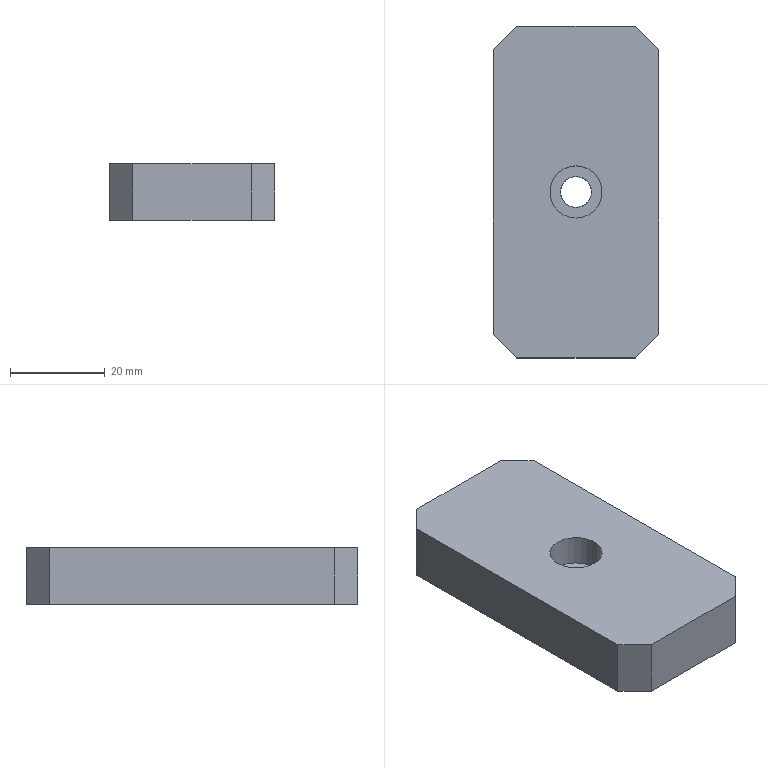Part | STEP file | P011002NM03-000 | 1 solid | 13 faces | box 35 x 70 x 12 mm | volume 28000 mm3 | plane 11 | cylinder 2 | commonest cylinder face diameters 6.5 x1 11 x1
STEP:
#1=CARTESIAN_POINT('',(0.,0.,0.));
#2=DIRECTION('',(0.,0.,1.));
#3=DIRECTION('',(1.,0.,0.));
#4=AXIS2_PLACEMENT_3D('',#1,#2,#3);
#5=CARTESIAN_POINT('',(-207.5,157.5,9.));
#6=VERTEX_POINT('',#5);
#7=CARTESIAN_POINT('',(-232.5,157.5,9.));
#8=VERTEX_POINT('',#7);
#9=CARTESIAN_POINT('',(-220.,157.5,9.));
#10=DIRECTION('',(-1.,0.,0.));
#11=VECTOR('',#10,1.);
#12=LINE('',#9,#11);
#13=CARTESIAN_POINT('',(-220.,157.5,6.));
#14=DIRECTION('',(0.,-1.,0.));
#15=DIRECTION('',(0.,0.,-1.));
#16=AXIS2_PLACEMENT_3D('',#13,#14,#15);
#17=PLANE('',#16);
#18=CARTESIAN_POINT('',(-3.,0.));
#19=DIRECTION('',(0.,-1.));
#20=VECTOR('',#19,1.);
#21=LINE('',#18,#20);
#22=(GEOMETRIC_REPRESENTATION_CONTEXT(2)PARAMETRIC_REPRESENTATION_CONTEXT()REPRESENTATION_CONTEXT('',''));
#23=DEFINITIONAL_REPRESENTATION('',(#21),#22);
#24=PCURVE('',#17,#23);
#25=CARTESIAN_POINT('',(178.,-325.,9.));
#26=DIRECTION('',(0.,0.,1.));
#27=DIRECTION('',(1.,0.,0.));
#28=AXIS2_PLACEMENT_3D('',#25,#26,#27);
#29=PLANE('',#28);
#30=CARTESIAN_POINT('',(-398.,482.5));
#31=DIRECTION('',(-1.,0.));
#32=VECTOR('',#31,1.);
#33=LINE('',#30,#32);
#34=(GEOMETRIC_REPRESENTATION_CONTEXT(2)PARAMETRIC_REPRESENTATION_CONTEXT()REPRESENTATION_CONTEXT('',''));
#35=DEFINITIONAL_REPRESENTATION('',(#33),#34);
#36=PCURVE('',#29,#35);
#37=SURFACE_CURVE('',#12,(#24,#36),.PCURVE_S1.);
#38=EDGE_CURVE('',#6,#8,#37,.T.);
#39=ORIENTED_EDGE('',*,*,#38,.F.);
#40=CARTESIAN_POINT('',(-207.5,157.5,21.));
#41=VERTEX_POINT('',#40);
#42=CARTESIAN_POINT('',(-207.5,157.5,6.));
#43=DIRECTION('',(0.,0.,1.));
#44=VECTOR('',#43,1.);
#45=LINE('',#42,#44);
#46=CARTESIAN_POINT('',(0.,12.5));
#47=DIRECTION('',(-1.,0.));
#48=VECTOR('',#47,1.);
#49=LINE('',#46,#48);
#50=(GEOMETRIC_REPRESENTATION_CONTEXT(2)PARAMETRIC_REPRESENTATION_CONTEXT()REPRESENTATION_CONTEXT('',''));
#51=DEFINITIONAL_REPRESENTATION('',(#49),#50);
#52=PCURVE('',#17,#51);
#53=CARTESIAN_POINT('',(-202.5,162.5,6.));
#54=DIRECTION('',(-0.7071,0.7071,0.));
#55=DIRECTION('',(-0.7071,-0.7071,0.));
#56=AXIS2_PLACEMENT_3D('',#53,#54,#55);
#57=PLANE('',#56);
#58=CARTESIAN_POINT('',(7.071,0.));
#59=DIRECTION('',(0.,1.));
#60=VECTOR('',#59,1.);
#61=LINE('',#58,#60);
#62=(GEOMETRIC_REPRESENTATION_CONTEXT(2)PARAMETRIC_REPRESENTATION_CONTEXT()REPRESENTATION_CONTEXT('',''));
#63=DEFINITIONAL_REPRESENTATION('',(#61),#62);
#64=PCURVE('',#57,#63);
#65=SURFACE_CURVE('',#45,(#52,#64),.PCURVE_S1.);
#66=EDGE_CURVE('',#6,#41,#65,.T.);
#67=ORIENTED_EDGE('',*,*,#66,.T.);
#68=CARTESIAN_POINT('',(-232.5,157.5,21.));
#69=VERTEX_POINT('',#68);
#70=CARTESIAN_POINT('',(-220.,157.5,21.));
#71=DIRECTION('',(-1.,0.,0.));
#72=VECTOR('',#71,1.);
#73=LINE('',#70,#72);
#74=CARTESIAN_POINT('',(-15.,0.));
#75=DIRECTION('',(0.,-1.));
#76=VECTOR('',#75,1.);
#77=LINE('',#74,#76);
#78=(GEOMETRIC_REPRESENTATION_CONTEXT(2)PARAMETRIC_REPRESENTATION_CONTEXT()REPRESENTATION_CONTEXT('',''));
#79=DEFINITIONAL_REPRESENTATION('',(#77),#78);
#80=PCURVE('',#17,#79);
#81=CARTESIAN_POINT('',(-205.,185.,21.));
#82=DIRECTION('',(0.,0.,1.));
#83=DIRECTION('',(1.,0.,0.));
#84=AXIS2_PLACEMENT_3D('',#81,#82,#83);
#85=PLANE('',#84);
#86=CARTESIAN_POINT('',(-15.,-27.5));
#87=DIRECTION('',(-1.,0.));
#88=VECTOR('',#87,1.);
#89=LINE('',#86,#88);
#90=(GEOMETRIC_REPRESENTATION_CONTEXT(2)PARAMETRIC_REPRESENTATION_CONTEXT()REPRESENTATION_CONTEXT('',''));
#91=DEFINITIONAL_REPRESENTATION('',(#89),#90);
#92=PCURVE('',#85,#91);
#93=SURFACE_CURVE('',#73,(#80,#92),.PCURVE_S1.);
#94=EDGE_CURVE('',#41,#69,#93,.T.);
#95=ORIENTED_EDGE('',*,*,#94,.T.);
#96=CARTESIAN_POINT('',(-232.5,157.5,6.));
#97=DIRECTION('',(0.,0.,-1.));
#98=VECTOR('',#97,1.);
#99=LINE('',#96,#98);
#100=CARTESIAN_POINT('',(0.,-12.5));
#101=DIRECTION('',(1.,0.));
#102=VECTOR('',#101,1.);
#103=LINE('',#100,#102);
#104=(GEOMETRIC_REPRESENTATION_CONTEXT(2)PARAMETRIC_REPRESENTATION_CONTEXT()REPRESENTATION_CONTEXT('',''));
#105=DEFINITIONAL_REPRESENTATION('',(#103),#104);
#106=PCURVE('',#17,#105);
#107=CARTESIAN_POINT('',(-232.5,157.5,6.));
#108=DIRECTION('',(0.7071,0.7071,0.));
#109=DIRECTION('',(-0.7071,0.7071,0.));
#110=AXIS2_PLACEMENT_3D('',#107,#108,#109);
#111=PLANE('',#110);
#112=CARTESIAN_POINT('',(0.,0.));
#113=DIRECTION('',(0.,-1.));
#114=VECTOR('',#113,1.);
#115=LINE('',#112,#114);
#116=(GEOMETRIC_REPRESENTATION_CONTEXT(2)PARAMETRIC_REPRESENTATION_CONTEXT()REPRESENTATION_CONTEXT('',''));
#117=DEFINITIONAL_REPRESENTATION('',(#115),#116);
#118=PCURVE('',#111,#117);
#119=SURFACE_CURVE('',#99,(#106,#118),.PCURVE_S1.);
#120=EDGE_CURVE('',#69,#8,#119,.T.);
#121=ORIENTED_EDGE('',*,*,#120,.T.);
#122=EDGE_LOOP('',(#39,#67,#95,#121));
#123=FACE_BOUND('',#122,.T.);
#124=ADVANCED_FACE('',(#123),#17,.T.);
#125=CARTESIAN_POINT('',(-202.5,222.5,9.));
#126=VERTEX_POINT('',#125);
#127=CARTESIAN_POINT('',(-202.5,162.5,9.));
#128=VERTEX_POINT('',#127);
#129=CARTESIAN_POINT('',(-202.5,192.5,9.));
#130=DIRECTION('',(0.,-1.,0.));
#131=VECTOR('',#130,1.);
#132=LINE('',#129,#131);
#133=CARTESIAN_POINT('',(-202.5,192.5,6.));
#134=DIRECTION('',(1.,0.,0.));
#135=DIRECTION('',(0.,0.,-1.));
#136=AXIS2_PLACEMENT_3D('',#133,#134,#135);
#137=PLANE('',#136);
#138=CARTESIAN_POINT('',(-3.,0.));
#139=DIRECTION('',(0.,-1.));
#140=VECTOR('',#139,1.);
#141=LINE('',#138,#140);
#142=(GEOMETRIC_REPRESENTATION_CONTEXT(2)PARAMETRIC_REPRESENTATION_CONTEXT()REPRESENTATION_CONTEXT('',''));
#143=DEFINITIONAL_REPRESENTATION('',(#141),#142);
#144=PCURVE('',#137,#143);
#145=CARTESIAN_POINT('',(-380.5,517.5));
#146=DIRECTION('',(0.,-1.));
#147=VECTOR('',#146,1.);
#148=LINE('',#145,#147);
#149=(GEOMETRIC_REPRESENTATION_CONTEXT(2)PARAMETRIC_REPRESENTATION_CONTEXT()REPRESENTATION_CONTEXT('',''));
#150=DEFINITIONAL_REPRESENTATION('',(#148),#149);
#151=PCURVE('',#29,#150);
#152=SURFACE_CURVE('',#132,(#144,#151),.PCURVE_S1.);
#153=EDGE_CURVE('',#126,#128,#152,.T.);
#154=ORIENTED_EDGE('',*,*,#153,.F.);
#155=CARTESIAN_POINT('',(-202.5,222.5,21.));
#156=VERTEX_POINT('',#155);
#157=CARTESIAN_POINT('',(-202.5,222.5,6.));
#158=DIRECTION('',(0.,0.,1.));
#159=VECTOR('',#158,1.);
#160=LINE('',#157,#159);
#161=CARTESIAN_POINT('',(0.,30.));
#162=DIRECTION('',(-1.,0.));
#163=VECTOR('',#162,1.);
#164=LINE('',#161,#163);
#165=(GEOMETRIC_REPRESENTATION_CONTEXT(2)PARAMETRIC_REPRESENTATION_CONTEXT()REPRESENTATION_CONTEXT('',''));
#166=DEFINITIONAL_REPRESENTATION('',(#164),#165);
#167=PCURVE('',#137,#166);
#168=CARTESIAN_POINT('',(-207.5,227.5,6.));
#169=DIRECTION('',(-0.7071,-0.7071,0.));
#170=DIRECTION('',(0.7071,-0.7071,0.));
#171=AXIS2_PLACEMENT_3D('',#168,#169,#170);
#172=PLANE('',#171);
#173=CARTESIAN_POINT('',(7.071,0.));
#174=DIRECTION('',(0.,1.));
#175=VECTOR('',#174,1.);
#176=LINE('',#173,#175);
#177=(GEOMETRIC_REPRESENTATION_CONTEXT(2)PARAMETRIC_REPRESENTATION_CONTEXT()REPRESENTATION_CONTEXT('',''));
#178=DEFINITIONAL_REPRESENTATION('',(#176),#177);
#179=PCURVE('',#172,#178);
#180=SURFACE_CURVE('',#160,(#167,#179),.PCURVE_S1.);
#181=EDGE_CURVE('',#126,#156,#180,.T.);
#182=ORIENTED_EDGE('',*,*,#181,.T.);
#183=CARTESIAN_POINT('',(-202.5,162.5,21.));
#184=VERTEX_POINT('',#183);
#185=CARTESIAN_POINT('',(-202.5,192.5,21.));
#186=DIRECTION('',(0.,-1.,0.));
#187=VECTOR('',#186,1.);
#188=LINE('',#185,#187);
#189=CARTESIAN_POINT('',(-15.,0.));
#190=DIRECTION('',(0.,-1.));
#191=VECTOR('',#190,1.);
#192=LINE('',#189,#191);
#193=(GEOMETRIC_REPRESENTATION_CONTEXT(2)PARAMETRIC_REPRESENTATION_CONTEXT()REPRESENTATION_CONTEXT('',''));
#194=DEFINITIONAL_REPRESENTATION('',(#192),#193);
#195=PCURVE('',#137,#194);
#196=CARTESIAN_POINT('',(2.5,7.5));
#197=DIRECTION('',(0.,-1.));
#198=VECTOR('',#197,1.);
#199=LINE('',#196,#198);
#200=(GEOMETRIC_REPRESENTATION_CONTEXT(2)PARAMETRIC_REPRESENTATION_CONTEXT()REPRESENTATION_CONTEXT('',''));
#201=DEFINITIONAL_REPRESENTATION('',(#199),#200);
#202=PCURVE('',#85,#201);
#203=SURFACE_CURVE('',#188,(#195,#202),.PCURVE_S1.);
#204=EDGE_CURVE('',#156,#184,#203,.T.);
#205=ORIENTED_EDGE('',*,*,#204,.T.);
#206=CARTESIAN_POINT('',(-202.5,162.5,6.));
#207=DIRECTION('',(0.,0.,-1.));
#208=VECTOR('',#207,1.);
#209=LINE('',#206,#208);
#210=CARTESIAN_POINT('',(0.,-30.));
#211=DIRECTION('',(1.,0.));
#212=VECTOR('',#211,1.);
#213=LINE('',#210,#212);
#214=(GEOMETRIC_REPRESENTATION_CONTEXT(2)PARAMETRIC_REPRESENTATION_CONTEXT()REPRESENTATION_CONTEXT('',''));
#215=DEFINITIONAL_REPRESENTATION('',(#213),#214);
#216=PCURVE('',#137,#215);
#217=CARTESIAN_POINT('',(0.,0.));
#218=DIRECTION('',(0.,-1.));
#219=VECTOR('',#218,1.);
#220=LINE('',#217,#219);
#221=(GEOMETRIC_REPRESENTATION_CONTEXT(2)PARAMETRIC_REPRESENTATION_CONTEXT()REPRESENTATION_CONTEXT('',''));
#222=DEFINITIONAL_REPRESENTATION('',(#220),#221);
#223=PCURVE('',#57,#222);
#224=SURFACE_CURVE('',#209,(#216,#223),.PCURVE_S1.);
#225=EDGE_CURVE('',#184,#128,#224,.T.);
#226=ORIENTED_EDGE('',*,*,#225,.T.);
#227=EDGE_LOOP('',(#154,#182,#205,#226));
#228=FACE_BOUND('',#227,.T.);
#229=ADVANCED_FACE('',(#228),#137,.T.);
#230=CARTESIAN_POINT('',(-232.5,227.5,9.));
#231=VERTEX_POINT('',#230);
#232=CARTESIAN_POINT('',(-207.5,227.5,9.));
#233=VERTEX_POINT('',#232);
#234=CARTESIAN_POINT('',(-220.,227.5,9.));
#235=DIRECTION('',(1.,0.,0.));
#236=VECTOR('',#235,1.);
#237=LINE('',#234,#236);
#238=CARTESIAN_POINT('',(-220.,227.5,6.));
#239=DIRECTION('',(0.,1.,0.));
#240=DIRECTION('',(0.,0.,1.));
#241=AXIS2_PLACEMENT_3D('',#238,#239,#240);
#242=PLANE('',#241);
#243=CARTESIAN_POINT('',(3.,0.));
#244=DIRECTION('',(0.,1.));
#245=VECTOR('',#244,1.);
#246=LINE('',#243,#245);
#247=(GEOMETRIC_REPRESENTATION_CONTEXT(2)PARAMETRIC_REPRESENTATION_CONTEXT()REPRESENTATION_CONTEXT('',''));
#248=DEFINITIONAL_REPRESENTATION('',(#246),#247);
#249=PCURVE('',#242,#248);
#250=CARTESIAN_POINT('',(-398.,552.5));
#251=DIRECTION('',(1.,0.));
#252=VECTOR('',#251,1.);
#253=LINE('',#250,#252);
#254=(GEOMETRIC_REPRESENTATION_CONTEXT(2)PARAMETRIC_REPRESENTATION_CONTEXT()REPRESENTATION_CONTEXT('',''));
#255=DEFINITIONAL_REPRESENTATION('',(#253),#254);
#256=PCURVE('',#29,#255);
#257=SURFACE_CURVE('',#237,(#249,#256),.PCURVE_S1.);
#258=EDGE_CURVE('',#231,#233,#257,.T.);
#259=ORIENTED_EDGE('',*,*,#258,.F.);
#260=CARTESIAN_POINT('',(-232.5,227.5,21.));
#261=VERTEX_POINT('',#260);
#262=CARTESIAN_POINT('',(-232.5,227.5,6.));
#263=DIRECTION('',(0.,0.,1.));
#264=VECTOR('',#263,1.);
#265=LINE('',#262,#264);
#266=CARTESIAN_POINT('',(0.,-12.5));
#267=DIRECTION('',(1.,0.));
#268=VECTOR('',#267,1.);
#269=LINE('',#266,#268);
#270=(GEOMETRIC_REPRESENTATION_CONTEXT(2)PARAMETRIC_REPRESENTATION_CONTEXT()REPRESENTATION_CONTEXT('',''));
#271=DEFINITIONAL_REPRESENTATION('',(#269),#270);
#272=PCURVE('',#242,#271);
#273=CARTESIAN_POINT('',(-237.5,222.5,6.));
#274=DIRECTION('',(0.7071,-0.7071,0.));
#275=DIRECTION('',(0.7071,0.7071,0.));
#276=AXIS2_PLACEMENT_3D('',#273,#274,#275);
#277=PLANE('',#276);
#278=CARTESIAN_POINT('',(7.071,0.));
#279=DIRECTION('',(0.,1.));
#280=VECTOR('',#279,1.);
#281=LINE('',#278,#280);
#282=(GEOMETRIC_REPRESENTATION_CONTEXT(2)PARAMETRIC_REPRESENTATION_CONTEXT()REPRESENTATION_CONTEXT('',''));
#283=DEFINITIONAL_REPRESENTATION('',(#281),#282);
#284=PCURVE('',#277,#283);
#285=SURFACE_CURVE('',#265,(#272,#284),.PCURVE_S1.);
#286=EDGE_CURVE('',#231,#261,#285,.T.);
#287=ORIENTED_EDGE('',*,*,#286,.T.);
#288=CARTESIAN_POINT('',(-207.5,227.5,21.));
#289=VERTEX_POINT('',#288);
#290=CARTESIAN_POINT('',(-220.,227.5,21.));
#291=DIRECTION('',(1.,0.,0.));
#292=VECTOR('',#291,1.);
#293=LINE('',#290,#292);
#294=CARTESIAN_POINT('',(15.,0.));
#295=DIRECTION('',(0.,1.));
#296=VECTOR('',#295,1.);
#297=LINE('',#294,#296);
#298=(GEOMETRIC_REPRESENTATION_CONTEXT(2)PARAMETRIC_REPRESENTATION_CONTEXT()REPRESENTATION_CONTEXT('',''));
#299=DEFINITIONAL_REPRESENTATION('',(#297),#298);
#300=PCURVE('',#242,#299);
#301=CARTESIAN_POINT('',(-15.,42.5));
#302=DIRECTION('',(1.,0.));
#303=VECTOR('',#302,1.);
#304=LINE('',#301,#303);
#305=(GEOMETRIC_REPRESENTATION_CONTEXT(2)PARAMETRIC_REPRESENTATION_CONTEXT()REPRESENTATION_CONTEXT('',''));
#306=DEFINITIONAL_REPRESENTATION('',(#304),#305);
#307=PCURVE('',#85,#306);
#308=SURFACE_CURVE('',#293,(#300,#307),.PCURVE_S1.);
#309=EDGE_CURVE('',#261,#289,#308,.T.);
#310=ORIENTED_EDGE('',*,*,#309,.T.);
#311=CARTESIAN_POINT('',(-207.5,227.5,6.));
#312=DIRECTION('',(0.,0.,-1.));
#313=VECTOR('',#312,1.);
#314=LINE('',#311,#313);
#315=CARTESIAN_POINT('',(0.,12.5));
#316=DIRECTION('',(-1.,0.));
#317=VECTOR('',#316,1.);
#318=LINE('',#315,#317);
#319=(GEOMETRIC_REPRESENTATION_CONTEXT(2)PARAMETRIC_REPRESENTATION_CONTEXT()REPRESENTATION_CONTEXT('',''));
#320=DEFINITIONAL_REPRESENTATION('',(#318),#319);
#321=PCURVE('',#242,#320);
#322=CARTESIAN_POINT('',(0.,0.));
#323=DIRECTION('',(0.,-1.));
#324=VECTOR('',#323,1.);
#325=LINE('',#322,#324);
#326=(GEOMETRIC_REPRESENTATION_CONTEXT(2)PARAMETRIC_REPRESENTATION_CONTEXT()REPRESENTATION_CONTEXT('',''));
#327=DEFINITIONAL_REPRESENTATION('',(#325),#326);
#328=PCURVE('',#172,#327);
#329=SURFACE_CURVE('',#314,(#321,#328),.PCURVE_S1.);
#330=EDGE_CURVE('',#289,#233,#329,.T.);
#331=ORIENTED_EDGE('',*,*,#330,.T.);
#332=EDGE_LOOP('',(#259,#287,#310,#331));
#333=FACE_BOUND('',#332,.T.);
#334=ADVANCED_FACE('',(#333),#242,.T.);
#335=CARTESIAN_POINT('',(-220.,187.,21.));
#336=VERTEX_POINT('',#335);
#337=CARTESIAN_POINT('',(-220.,192.5,21.));
#338=DIRECTION('',(0.,0.,1.));
#339=DIRECTION('',(0.,-1.,0.));
#340=AXIS2_PLACEMENT_3D('',#337,#338,#339);
#341=CIRCLE('',#340,5.5);
#342=CARTESIAN_POINT('',(-15.,7.5));
#343=DIRECTION('',(0.,-1.));
#344=AXIS2_PLACEMENT_2D('',#342,#343);
#345=CIRCLE('',#344,5.5);
#346=(GEOMETRIC_REPRESENTATION_CONTEXT(2)PARAMETRIC_REPRESENTATION_CONTEXT()REPRESENTATION_CONTEXT('',''));
#347=DEFINITIONAL_REPRESENTATION('',(#345),#346);
#348=PCURVE('',#85,#347);
#349=CARTESIAN_POINT('',(-220.,192.5,22.));
#350=DIRECTION('',(0.,0.,1.));
#351=DIRECTION('',(0.,-1.,0.));
#352=AXIS2_PLACEMENT_3D('',#349,#350,#351);
#353=CYLINDRICAL_SURFACE('',#352,5.5);
#354=CARTESIAN_POINT('',(0.,-1.));
#355=DIRECTION('',(1.,0.));
#356=VECTOR('',#355,1.);
#357=LINE('',#354,#356);
#358=(GEOMETRIC_REPRESENTATION_CONTEXT(2)PARAMETRIC_REPRESENTATION_CONTEXT()REPRESENTATION_CONTEXT('',''));
#359=DEFINITIONAL_REPRESENTATION('',(#357),#358);
#360=PCURVE('',#353,#359);
#361=SURFACE_CURVE('',#341,(#348,#360),.PCURVE_S1.);
#362=EDGE_CURVE('',#336,#336,#361,.T.);
#363=ORIENTED_EDGE('',*,*,#362,.F.);
#364=EDGE_LOOP('',(#363));
#365=FACE_BOUND('',#364,.T.);
#366=ORIENTED_EDGE('',*,*,#309,.F.);
#367=CARTESIAN_POINT('',(-237.5,222.5,21.));
#368=VERTEX_POINT('',#367);
#369=CARTESIAN_POINT('',(-241.25,218.75,21.));
#370=DIRECTION('',(-0.7071,-0.7071,0.));
#371=VECTOR('',#370,1.);
#372=LINE('',#369,#371);
#373=CARTESIAN_POINT('',(-36.25,33.75));
#374=DIRECTION('',(-0.7071,-0.7071));
#375=VECTOR('',#374,1.);
#376=LINE('',#373,#375);
#377=(GEOMETRIC_REPRESENTATION_CONTEXT(2)PARAMETRIC_REPRESENTATION_CONTEXT()REPRESENTATION_CONTEXT('',''));
#378=DEFINITIONAL_REPRESENTATION('',(#376),#377);
#379=PCURVE('',#85,#378);
#380=CARTESIAN_POINT('',(-5.303,15.));
#381=DIRECTION('',(-1.,0.));
#382=VECTOR('',#381,1.);
#383=LINE('',#380,#382);
#384=(GEOMETRIC_REPRESENTATION_CONTEXT(2)PARAMETRIC_REPRESENTATION_CONTEXT()REPRESENTATION_CONTEXT('',''));
#385=DEFINITIONAL_REPRESENTATION('',(#383),#384);
#386=PCURVE('',#277,#385);
#387=SURFACE_CURVE('',#372,(#379,#386),.PCURVE_S1.);
#388=EDGE_CURVE('',#261,#368,#387,.T.);
#389=ORIENTED_EDGE('',*,*,#388,.T.);
#390=CARTESIAN_POINT('',(-237.5,162.5,21.));
#391=VERTEX_POINT('',#390);
#392=CARTESIAN_POINT('',(-237.5,192.5,21.));
#393=DIRECTION('',(0.,1.,0.));
#394=VECTOR('',#393,1.);
#395=LINE('',#392,#394);
#396=CARTESIAN_POINT('',(-32.5,7.5));
#397=DIRECTION('',(0.,1.));
#398=VECTOR('',#397,1.);
#399=LINE('',#396,#398);
#400=(GEOMETRIC_REPRESENTATION_CONTEXT(2)PARAMETRIC_REPRESENTATION_CONTEXT()REPRESENTATION_CONTEXT('',''));
#401=DEFINITIONAL_REPRESENTATION('',(#399),#400);
#402=PCURVE('',#85,#401);
#403=CARTESIAN_POINT('',(-237.5,192.5,6.));
#404=DIRECTION('',(-1.,0.,0.));
#405=DIRECTION('',(0.,0.,1.));
#406=AXIS2_PLACEMENT_3D('',#403,#404,#405);
#407=PLANE('',#406);
#408=CARTESIAN_POINT('',(15.,0.));
#409=DIRECTION('',(0.,1.));
#410=VECTOR('',#409,1.);
#411=LINE('',#408,#410);
#412=(GEOMETRIC_REPRESENTATION_CONTEXT(2)PARAMETRIC_REPRESENTATION_CONTEXT()REPRESENTATION_CONTEXT('',''));
#413=DEFINITIONAL_REPRESENTATION('',(#411),#412);
#414=PCURVE('',#407,#413);
#415=SURFACE_CURVE('',#395,(#402,#414),.PCURVE_S1.);
#416=EDGE_CURVE('',#391,#368,#415,.T.);
#417=ORIENTED_EDGE('',*,*,#416,.F.);
#418=CARTESIAN_POINT('',(-233.75,158.75,21.));
#419=DIRECTION('',(0.7071,-0.7071,0.));
#420=VECTOR('',#419,1.);
#421=LINE('',#418,#420);
#422=CARTESIAN_POINT('',(-28.75,-26.25));
#423=DIRECTION('',(0.7071,-0.7071));
#424=VECTOR('',#423,1.);
#425=LINE('',#422,#424);
#426=(GEOMETRIC_REPRESENTATION_CONTEXT(2)PARAMETRIC_REPRESENTATION_CONTEXT()REPRESENTATION_CONTEXT('',''));
#427=DEFINITIONAL_REPRESENTATION('',(#425),#426);
#428=PCURVE('',#85,#427);
#429=CARTESIAN_POINT('',(1.768,15.));
#430=DIRECTION('',(-1.,0.));
#431=VECTOR('',#430,1.);
#432=LINE('',#429,#431);
#433=(GEOMETRIC_REPRESENTATION_CONTEXT(2)PARAMETRIC_REPRESENTATION_CONTEXT()REPRESENTATION_CONTEXT('',''));
#434=DEFINITIONAL_REPRESENTATION('',(#432),#433);
#435=PCURVE('',#111,#434);
#436=SURFACE_CURVE('',#421,(#428,#435),.PCURVE_S1.);
#437=EDGE_CURVE('',#391,#69,#436,.T.);
#438=ORIENTED_EDGE('',*,*,#437,.T.);
#439=ORIENTED_EDGE('',*,*,#94,.F.);
#440=CARTESIAN_POINT('',(-191.25,173.75,21.));
#441=DIRECTION('',(0.7071,0.7071,0.));
#442=VECTOR('',#441,1.);
#443=LINE('',#440,#442);
#444=CARTESIAN_POINT('',(13.75,-11.25));
#445=DIRECTION('',(0.7071,0.7071));
#446=VECTOR('',#445,1.);
#447=LINE('',#444,#446);
#448=(GEOMETRIC_REPRESENTATION_CONTEXT(2)PARAMETRIC_REPRESENTATION_CONTEXT()REPRESENTATION_CONTEXT('',''));
#449=DEFINITIONAL_REPRESENTATION('',(#447),#448);
#450=PCURVE('',#85,#449);
#451=CARTESIAN_POINT('',(-15.91,15.));
#452=DIRECTION('',(-1.,0.));
#453=VECTOR('',#452,1.);
#454=LINE('',#451,#453);
#455=(GEOMETRIC_REPRESENTATION_CONTEXT(2)PARAMETRIC_REPRESENTATION_CONTEXT()REPRESENTATION_CONTEXT('',''));
#456=DEFINITIONAL_REPRESENTATION('',(#454),#455);
#457=PCURVE('',#57,#456);
#458=SURFACE_CURVE('',#443,(#450,#457),.PCURVE_S1.);
#459=EDGE_CURVE('',#41,#184,#458,.T.);
#460=ORIENTED_EDGE('',*,*,#459,.T.);
#461=ORIENTED_EDGE('',*,*,#204,.F.);
#462=CARTESIAN_POINT('',(-183.75,203.75,21.));
#463=DIRECTION('',(-0.7071,0.7071,0.));
#464=VECTOR('',#463,1.);
#465=LINE('',#462,#464);
#466=CARTESIAN_POINT('',(21.25,18.75));
#467=DIRECTION('',(-0.7071,0.7071));
#468=VECTOR('',#467,1.);
#469=LINE('',#466,#468);
#470=(GEOMETRIC_REPRESENTATION_CONTEXT(2)PARAMETRIC_REPRESENTATION_CONTEXT()REPRESENTATION_CONTEXT('',''));
#471=DEFINITIONAL_REPRESENTATION('',(#469),#470);
#472=PCURVE('',#85,#471);
#473=CARTESIAN_POINT('',(33.588,15.));
#474=DIRECTION('',(-1.,0.));
#475=VECTOR('',#474,1.);
#476=LINE('',#473,#475);
#477=(GEOMETRIC_REPRESENTATION_CONTEXT(2)PARAMETRIC_REPRESENTATION_CONTEXT()REPRESENTATION_CONTEXT('',''));
#478=DEFINITIONAL_REPRESENTATION('',(#476),#477);
#479=PCURVE('',#172,#478);
#480=SURFACE_CURVE('',#465,(#472,#479),.PCURVE_S1.);
#481=EDGE_CURVE('',#156,#289,#480,.T.);
#482=ORIENTED_EDGE('',*,*,#481,.T.);
#483=EDGE_LOOP('',(#366,#389,#417,#438,#439,#460,#461,#482));
#484=FACE_BOUND('',#483,.T.);
#485=ADVANCED_FACE('',(#365,#484),#85,.T.);
#486=CARTESIAN_POINT('',(-237.5,162.5,9.));
#487=VERTEX_POINT('',#486);
#488=CARTESIAN_POINT('',(-237.5,222.5,9.));
#489=VERTEX_POINT('',#488);
#490=CARTESIAN_POINT('',(-237.5,192.5,9.));
#491=DIRECTION('',(0.,1.,0.));
#492=VECTOR('',#491,1.);
#493=LINE('',#490,#492);
#494=CARTESIAN_POINT('',(3.,0.));
#495=DIRECTION('',(0.,1.));
#496=VECTOR('',#495,1.);
#497=LINE('',#494,#496);
#498=(GEOMETRIC_REPRESENTATION_CONTEXT(2)PARAMETRIC_REPRESENTATION_CONTEXT()REPRESENTATION_CONTEXT('',''));
#499=DEFINITIONAL_REPRESENTATION('',(#497),#498);
#500=PCURVE('',#407,#499);
#501=CARTESIAN_POINT('',(-415.5,517.5));
#502=DIRECTION('',(0.,1.));
#503=VECTOR('',#502,1.);
#504=LINE('',#501,#503);
#505=(GEOMETRIC_REPRESENTATION_CONTEXT(2)PARAMETRIC_REPRESENTATION_CONTEXT()REPRESENTATION_CONTEXT('',''));
#506=DEFINITIONAL_REPRESENTATION('',(#504),#505);
#507=PCURVE('',#29,#506);
#508=SURFACE_CURVE('',#493,(#500,#507),.PCURVE_S1.);
#509=EDGE_CURVE('',#487,#489,#508,.T.);
#510=ORIENTED_EDGE('',*,*,#509,.F.);
#511=CARTESIAN_POINT('',(-237.5,162.5,6.));
#512=DIRECTION('',(0.,0.,1.));
#513=VECTOR('',#512,1.);
#514=LINE('',#511,#513);
#515=CARTESIAN_POINT('',(0.,-30.));
#516=DIRECTION('',(1.,0.));
#517=VECTOR('',#516,1.);
#518=LINE('',#515,#517);
#519=(GEOMETRIC_REPRESENTATION_CONTEXT(2)PARAMETRIC_REPRESENTATION_CONTEXT()REPRESENTATION_CONTEXT('',''));
#520=DEFINITIONAL_REPRESENTATION('',(#518),#519);
#521=PCURVE('',#407,#520);
#522=CARTESIAN_POINT('',(7.071,0.));
#523=DIRECTION('',(0.,1.));
#524=VECTOR('',#523,1.);
#525=LINE('',#522,#524);
#526=(GEOMETRIC_REPRESENTATION_CONTEXT(2)PARAMETRIC_REPRESENTATION_CONTEXT()REPRESENTATION_CONTEXT('',''));
#527=DEFINITIONAL_REPRESENTATION('',(#525),#526);
#528=PCURVE('',#111,#527);
#529=SURFACE_CURVE('',#514,(#521,#528),.PCURVE_S1.);
#530=EDGE_CURVE('',#487,#391,#529,.T.);
#531=ORIENTED_EDGE('',*,*,#530,.T.);
#532=ORIENTED_EDGE('',*,*,#416,.T.);
#533=CARTESIAN_POINT('',(-237.5,222.5,6.));
#534=DIRECTION('',(0.,0.,-1.));
#535=VECTOR('',#534,1.);
#536=LINE('',#533,#535);
#537=CARTESIAN_POINT('',(0.,30.));
#538=DIRECTION('',(-1.,0.));
#539=VECTOR('',#538,1.);
#540=LINE('',#537,#539);
#541=(GEOMETRIC_REPRESENTATION_CONTEXT(2)PARAMETRIC_REPRESENTATION_CONTEXT()REPRESENTATION_CONTEXT('',''));
#542=DEFINITIONAL_REPRESENTATION('',(#540),#541);
#543=PCURVE('',#407,#542);
#544=CARTESIAN_POINT('',(0.,0.));
#545=DIRECTION('',(0.,-1.));
#546=VECTOR('',#545,1.);
#547=LINE('',#544,#546);
#548=(GEOMETRIC_REPRESENTATION_CONTEXT(2)PARAMETRIC_REPRESENTATION_CONTEXT()REPRESENTATION_CONTEXT('',''));
#549=DEFINITIONAL_REPRESENTATION('',(#547),#548);
#550=PCURVE('',#277,#549);
#551=SURFACE_CURVE('',#536,(#543,#550),.PCURVE_S1.);
#552=EDGE_CURVE('',#368,#489,#551,.T.);
#553=ORIENTED_EDGE('',*,*,#552,.T.);
#554=EDGE_LOOP('',(#510,#531,#532,#553));
#555=FACE_BOUND('',#554,.T.);
#556=ADVANCED_FACE('',(#555),#407,.T.);
#557=CARTESIAN_POINT('',(-237.5,222.5,9.));
#558=DIRECTION('',(0.7071,0.7071,0.));
#559=VECTOR('',#558,1.);
#560=LINE('',#557,#559);
#561=CARTESIAN_POINT('',(0.,3.));
#562=DIRECTION('',(1.,0.));
#563=VECTOR('',#562,1.);
#564=LINE('',#561,#563);
#565=(GEOMETRIC_REPRESENTATION_CONTEXT(2)PARAMETRIC_REPRESENTATION_CONTEXT()REPRESENTATION_CONTEXT('',''));
#566=DEFINITIONAL_REPRESENTATION('',(#564),#565);
#567=PCURVE('',#277,#566);
#568=CARTESIAN_POINT('',(-415.5,547.5));
#569=DIRECTION('',(0.7071,0.7071));
#570=VECTOR('',#569,1.);
#571=LINE('',#568,#570);
#572=(GEOMETRIC_REPRESENTATION_CONTEXT(2)PARAMETRIC_REPRESENTATION_CONTEXT()REPRESENTATION_CONTEXT('',''));
#573=DEFINITIONAL_REPRESENTATION('',(#571),#572);
#574=PCURVE('',#29,#573);
#575=SURFACE_CURVE('',#560,(#567,#574),.PCURVE_S1.);
#576=EDGE_CURVE('',#489,#231,#575,.T.);
#577=ORIENTED_EDGE('',*,*,#576,.F.);
#578=ORIENTED_EDGE('',*,*,#552,.F.);
#579=ORIENTED_EDGE('',*,*,#388,.F.);
#580=ORIENTED_EDGE('',*,*,#286,.F.);
#581=EDGE_LOOP('',(#577,#578,#579,#580));
#582=FACE_BOUND('',#581,.T.);
#583=ADVANCED_FACE('',(#582),#277,.F.);
#584=CARTESIAN_POINT('',(-232.5,157.5,9.));
#585=DIRECTION('',(-0.7071,0.7071,0.));
#586=VECTOR('',#585,1.);
#587=LINE('',#584,#586);
#588=CARTESIAN_POINT('',(0.,3.));
#589=DIRECTION('',(1.,0.));
#590=VECTOR('',#589,1.);
#591=LINE('',#588,#590);
#592=(GEOMETRIC_REPRESENTATION_CONTEXT(2)PARAMETRIC_REPRESENTATION_CONTEXT()REPRESENTATION_CONTEXT('',''));
#593=DEFINITIONAL_REPRESENTATION('',(#591),#592);
#594=PCURVE('',#111,#593);
#595=CARTESIAN_POINT('',(-410.5,482.5));
#596=DIRECTION('',(-0.7071,0.7071));
#597=VECTOR('',#596,1.);
#598=LINE('',#595,#597);
#599=(GEOMETRIC_REPRESENTATION_CONTEXT(2)PARAMETRIC_REPRESENTATION_CONTEXT()REPRESENTATION_CONTEXT('',''));
#600=DEFINITIONAL_REPRESENTATION('',(#598),#599);
#601=PCURVE('',#29,#600);
#602=SURFACE_CURVE('',#587,(#594,#601),.PCURVE_S1.);
#603=EDGE_CURVE('',#8,#487,#602,.T.);
#604=ORIENTED_EDGE('',*,*,#603,.F.);
#605=ORIENTED_EDGE('',*,*,#120,.F.);
#606=ORIENTED_EDGE('',*,*,#437,.F.);
#607=ORIENTED_EDGE('',*,*,#530,.F.);
#608=EDGE_LOOP('',(#604,#605,#606,#607));
#609=FACE_BOUND('',#608,.T.);
#610=ADVANCED_FACE('',(#609),#111,.F.);
#611=CARTESIAN_POINT('',(-207.5,227.5,9.));
#612=DIRECTION('',(0.7071,-0.7071,0.));
#613=VECTOR('',#612,1.);
#614=LINE('',#611,#613);
#615=CARTESIAN_POINT('',(0.,3.));
#616=DIRECTION('',(1.,0.));
#617=VECTOR('',#616,1.);
#618=LINE('',#615,#617);
#619=(GEOMETRIC_REPRESENTATION_CONTEXT(2)PARAMETRIC_REPRESENTATION_CONTEXT()REPRESENTATION_CONTEXT('',''));
#620=DEFINITIONAL_REPRESENTATION('',(#618),#619);
#621=PCURVE('',#172,#620);
#622=CARTESIAN_POINT('',(-385.5,552.5));
#623=DIRECTION('',(0.7071,-0.7071));
#624=VECTOR('',#623,1.);
#625=LINE('',#622,#624);
#626=(GEOMETRIC_REPRESENTATION_CONTEXT(2)PARAMETRIC_REPRESENTATION_CONTEXT()REPRESENTATION_CONTEXT('',''));
#627=DEFINITIONAL_REPRESENTATION('',(#625),#626);
#628=PCURVE('',#29,#627);
#629=SURFACE_CURVE('',#614,(#621,#628),.PCURVE_S1.);
#630=EDGE_CURVE('',#233,#126,#629,.T.);
#631=ORIENTED_EDGE('',*,*,#630,.F.);
#632=ORIENTED_EDGE('',*,*,#330,.F.);
#633=ORIENTED_EDGE('',*,*,#481,.F.);
#634=ORIENTED_EDGE('',*,*,#181,.F.);
#635=EDGE_LOOP('',(#631,#632,#633,#634));
#636=FACE_BOUND('',#635,.T.);
#637=ADVANCED_FACE('',(#636),#172,.F.);
#638=CARTESIAN_POINT('',(-202.5,162.5,9.));
#639=DIRECTION('',(-0.7071,-0.7071,0.));
#640=VECTOR('',#639,1.);
#641=LINE('',#638,#640);
#642=CARTESIAN_POINT('',(0.,3.));
#643=DIRECTION('',(1.,0.));
#644=VECTOR('',#643,1.);
#645=LINE('',#642,#644);
#646=(GEOMETRIC_REPRESENTATION_CONTEXT(2)PARAMETRIC_REPRESENTATION_CONTEXT()REPRESENTATION_CONTEXT('',''));
#647=DEFINITIONAL_REPRESENTATION('',(#645),#646);
#648=PCURVE('',#57,#647);
#649=CARTESIAN_POINT('',(-380.5,487.5));
#650=DIRECTION('',(-0.7071,-0.7071));
#651=VECTOR('',#650,1.);
#652=LINE('',#649,#651);
#653=(GEOMETRIC_REPRESENTATION_CONTEXT(2)PARAMETRIC_REPRESENTATION_CONTEXT()REPRESENTATION_CONTEXT('',''));
#654=DEFINITIONAL_REPRESENTATION('',(#652),#653);
#655=PCURVE('',#29,#654);
#656=SURFACE_CURVE('',#641,(#648,#655),.PCURVE_S1.);
#657=EDGE_CURVE('',#128,#6,#656,.T.);
#658=ORIENTED_EDGE('',*,*,#657,.F.);
#659=ORIENTED_EDGE('',*,*,#225,.F.);
#660=ORIENTED_EDGE('',*,*,#459,.F.);
#661=ORIENTED_EDGE('',*,*,#66,.F.);
#662=EDGE_LOOP('',(#658,#659,#660,#661));
#663=FACE_BOUND('',#662,.T.);
#664=ADVANCED_FACE('',(#663),#57,.F.);
#665=CARTESIAN_POINT('',(-216.75,192.5,9.));
#666=VERTEX_POINT('',#665);
#667=CARTESIAN_POINT('',(-220.,189.25,9.));
#668=VERTEX_POINT('',#667);
#669=CARTESIAN_POINT('',(-220.,192.5,9.));
#670=DIRECTION('',(0.,0.,1.));
#671=DIRECTION('',(1.,0.,0.));
#672=AXIS2_PLACEMENT_3D('',#669,#670,#671);
#673=CIRCLE('',#672,3.25);
#674=CARTESIAN_POINT('',(-398.,517.5));
#675=DIRECTION('',(1.,0.));
#676=AXIS2_PLACEMENT_2D('',#674,#675);
#677=CIRCLE('',#676,3.25);
#678=(GEOMETRIC_REPRESENTATION_CONTEXT(2)PARAMETRIC_REPRESENTATION_CONTEXT()REPRESENTATION_CONTEXT('',''));
#679=DEFINITIONAL_REPRESENTATION('',(#677),#678);
#680=PCURVE('',#29,#679);
#681=CARTESIAN_POINT('',(-220.,192.5,22.));
#682=DIRECTION('',(0.,0.,1.));
#683=DIRECTION('',(0.,-1.,0.));
#684=AXIS2_PLACEMENT_3D('',#681,#682,#683);
#685=CYLINDRICAL_SURFACE('',#684,3.25);
#686=CARTESIAN_POINT('',(1.571,-13.));
#687=DIRECTION('',(1.,0.));
#688=VECTOR('',#687,1.);
#689=LINE('',#686,#688);
#690=(GEOMETRIC_REPRESENTATION_CONTEXT(2)PARAMETRIC_REPRESENTATION_CONTEXT()REPRESENTATION_CONTEXT('',''));
#691=DEFINITIONAL_REPRESENTATION('',(#689),#690);
#692=PCURVE('',#685,#691);
#693=SURFACE_CURVE('',#673,(#680,#692),.PCURVE_S1.);
#694=EDGE_CURVE('',#666,#668,#693,.T.);
#695=ORIENTED_EDGE('',*,*,#694,.T.);
#696=CARTESIAN_POINT('',(-220.,192.5,9.));
#697=DIRECTION('',(0.,0.,1.));
#698=DIRECTION('',(1.,0.,0.));
#699=AXIS2_PLACEMENT_3D('',#696,#697,#698);
#700=CIRCLE('',#699,3.25);
#701=CARTESIAN_POINT('',(-398.,517.5));
#702=DIRECTION('',(1.,0.));
#703=AXIS2_PLACEMENT_2D('',#701,#702);
#704=CIRCLE('',#703,3.25);
#705=(GEOMETRIC_REPRESENTATION_CONTEXT(2)PARAMETRIC_REPRESENTATION_CONTEXT()REPRESENTATION_CONTEXT('',''));
#706=DEFINITIONAL_REPRESENTATION('',(#704),#705);
#707=PCURVE('',#29,#706);
#708=CARTESIAN_POINT('',(-4.712,-13.));
#709=DIRECTION('',(1.,0.));
#710=VECTOR('',#709,1.);
#711=LINE('',#708,#710);
#712=(GEOMETRIC_REPRESENTATION_CONTEXT(2)PARAMETRIC_REPRESENTATION_CONTEXT()REPRESENTATION_CONTEXT('',''));
#713=DEFINITIONAL_REPRESENTATION('',(#711),#712);
#714=PCURVE('',#685,#713);
#715=SURFACE_CURVE('',#700,(#707,#714),.PCURVE_S1.);
#716=EDGE_CURVE('',#668,#666,#715,.T.);
#717=ORIENTED_EDGE('',*,*,#716,.T.);
#718=EDGE_LOOP('',(#695,#717));
#719=FACE_BOUND('',#718,.T.);
#720=ORIENTED_EDGE('',*,*,#576,.T.);
#721=ORIENTED_EDGE('',*,*,#258,.T.);
#722=ORIENTED_EDGE('',*,*,#630,.T.);
#723=ORIENTED_EDGE('',*,*,#153,.T.);
#724=ORIENTED_EDGE('',*,*,#657,.T.);
#725=ORIENTED_EDGE('',*,*,#38,.T.);
#726=ORIENTED_EDGE('',*,*,#603,.T.);
#727=ORIENTED_EDGE('',*,*,#509,.T.);
#728=EDGE_LOOP('',(#720,#721,#722,#723,#724,#725,#726,#727));
#729=FACE_BOUND('',#728,.T.);
#730=ADVANCED_FACE('',(#719,#729),#29,.F.);
#731=CARTESIAN_POINT('',(-220.,189.25,14.5));
#732=VERTEX_POINT('',#731);
#733=CARTESIAN_POINT('',(-220.,192.5,14.5));
#734=DIRECTION('',(0.,0.,1.));
#735=DIRECTION('',(0.,-1.,0.));
#736=AXIS2_PLACEMENT_3D('',#733,#734,#735);
#737=CIRCLE('',#736,3.25);
#738=CARTESIAN_POINT('',(0.,-7.5));
#739=DIRECTION('',(1.,0.));
#740=VECTOR('',#739,1.);
#741=LINE('',#738,#740);
#742=(GEOMETRIC_REPRESENTATION_CONTEXT(2)PARAMETRIC_REPRESENTATION_CONTEXT()REPRESENTATION_CONTEXT('',''));
#743=DEFINITIONAL_REPRESENTATION('',(#741),#742);
#744=PCURVE('',#685,#743);
#745=CARTESIAN_POINT('',(-220.,192.5,14.5));
#746=DIRECTION('',(0.,0.,1.));
#747=DIRECTION('',(0.,-1.,0.));
#748=AXIS2_PLACEMENT_3D('',#745,#746,#747);
#749=PLANE('',#748);
#750=CARTESIAN_POINT('',(0.,0.));
#751=DIRECTION('',(1.,0.));
#752=AXIS2_PLACEMENT_2D('',#750,#751);
#753=CIRCLE('',#752,3.25);
#754=(GEOMETRIC_REPRESENTATION_CONTEXT(2)PARAMETRIC_REPRESENTATION_CONTEXT()REPRESENTATION_CONTEXT('',''));
#755=DEFINITIONAL_REPRESENTATION('',(#753),#754);
#756=PCURVE('',#749,#755);
#757=SURFACE_CURVE('',#737,(#744,#756),.PCURVE_S1.);
#758=EDGE_CURVE('',#732,#732,#757,.T.);
#759=ORIENTED_EDGE('',*,*,#758,.F.);
#760=CARTESIAN_POINT('',(-220.,189.25,9.));
#761=CARTESIAN_POINT('',(-220.,189.25,14.5));
#762=B_SPLINE_CURVE_WITH_KNOTS('',1,(#760,#761),.UNSPECIFIED.,.F.,.F.,(2,2),(-13.,-7.5),.PIECEWISE_BEZIER_KNOTS.);
#763=CARTESIAN_POINT('',(0.,0.));
#764=DIRECTION('',(0.,1.));
#765=VECTOR('',#764,1.);
#766=LINE('',#763,#765);
#767=(GEOMETRIC_REPRESENTATION_CONTEXT(2)PARAMETRIC_REPRESENTATION_CONTEXT()REPRESENTATION_CONTEXT('',''));
#768=DEFINITIONAL_REPRESENTATION('',(#766),#767);
#769=PCURVE('',#685,#768);
#770=CARTESIAN_POINT('',(6.283,0.));
#771=DIRECTION('',(0.,1.));
#772=VECTOR('',#771,1.);
#773=LINE('',#770,#772);
#774=(GEOMETRIC_REPRESENTATION_CONTEXT(2)PARAMETRIC_REPRESENTATION_CONTEXT()REPRESENTATION_CONTEXT('',''));
#775=DEFINITIONAL_REPRESENTATION('',(#773),#774);
#776=PCURVE('',#685,#775);
#777=SEAM_CURVE('',#762,(#769,#776),.PCURVE_S1.);
#778=EDGE_CURVE('',#668,#732,#777,.T.);
#779=ORIENTED_EDGE('',*,*,#778,.F.);
#780=ORIENTED_EDGE('',*,*,#716,.T.);
#781=ORIENTED_EDGE('',*,*,#694,.T.);
#782=ORIENTED_EDGE('',*,*,#778,.T.);
#783=EDGE_LOOP('',(#759,#779,#780,#781,#782));
#784=FACE_BOUND('',#783,.F.);
#785=ADVANCED_FACE('',(#784),#685,.F.);
#786=CARTESIAN_POINT('',(-220.,187.,14.5));
#787=VERTEX_POINT('',#786);
#788=CARTESIAN_POINT('',(-220.,192.5,14.5));
#789=DIRECTION('',(0.,0.,1.));
#790=DIRECTION('',(0.,-1.,0.));
#791=AXIS2_PLACEMENT_3D('',#788,#789,#790);
#792=CIRCLE('',#791,5.5);
#793=CARTESIAN_POINT('',(0.,0.));
#794=DIRECTION('',(1.,0.));
#795=AXIS2_PLACEMENT_2D('',#793,#794);
#796=CIRCLE('',#795,5.5);
#797=(GEOMETRIC_REPRESENTATION_CONTEXT(2)PARAMETRIC_REPRESENTATION_CONTEXT()REPRESENTATION_CONTEXT('',''));
#798=DEFINITIONAL_REPRESENTATION('',(#796),#797);
#799=PCURVE('',#749,#798);
#800=CARTESIAN_POINT('',(0.,-7.5));
#801=DIRECTION('',(1.,0.));
#802=VECTOR('',#801,1.);
#803=LINE('',#800,#802);
#804=(GEOMETRIC_REPRESENTATION_CONTEXT(2)PARAMETRIC_REPRESENTATION_CONTEXT()REPRESENTATION_CONTEXT('',''));
#805=DEFINITIONAL_REPRESENTATION('',(#803),#804);
#806=PCURVE('',#353,#805);
#807=SURFACE_CURVE('',#792,(#799,#806),.PCURVE_S1.);
#808=EDGE_CURVE('',#787,#787,#807,.T.);
#809=ORIENTED_EDGE('',*,*,#808,.T.);
#810=EDGE_LOOP('',(#809));
#811=FACE_BOUND('',#810,.T.);
#812=ORIENTED_EDGE('',*,*,#758,.F.);
#813=EDGE_LOOP('',(#812));
#814=FACE_BOUND('',#813,.T.);
#815=ADVANCED_FACE('',(#811,#814),#749,.T.);
#816=ORIENTED_EDGE('',*,*,#362,.F.);
#817=CARTESIAN_POINT('',(-220.,187.,14.5));
#818=CARTESIAN_POINT('',(-220.,187.,21.));
#819=B_SPLINE_CURVE_WITH_KNOTS('',1,(#817,#818),.UNSPECIFIED.,.F.,.F.,(2,2),(-7.5,-1.),.PIECEWISE_BEZIER_KNOTS.);
#820=CARTESIAN_POINT('',(0.,0.));
#821=DIRECTION('',(0.,1.));
#822=VECTOR('',#821,1.);
#823=LINE('',#820,#822);
#824=(GEOMETRIC_REPRESENTATION_CONTEXT(2)PARAMETRIC_REPRESENTATION_CONTEXT()REPRESENTATION_CONTEXT('',''));
#825=DEFINITIONAL_REPRESENTATION('',(#823),#824);
#826=PCURVE('',#353,#825);
#827=CARTESIAN_POINT('',(6.283,0.));
#828=DIRECTION('',(0.,1.));
#829=VECTOR('',#828,1.);
#830=LINE('',#827,#829);
#831=(GEOMETRIC_REPRESENTATION_CONTEXT(2)PARAMETRIC_REPRESENTATION_CONTEXT()REPRESENTATION_CONTEXT('',''));
#832=DEFINITIONAL_REPRESENTATION('',(#830),#831);
#833=PCURVE('',#353,#832);
#834=SEAM_CURVE('',#819,(#826,#833),.PCURVE_S1.);
#835=EDGE_CURVE('',#787,#336,#834,.T.);
#836=ORIENTED_EDGE('',*,*,#835,.F.);
#837=ORIENTED_EDGE('',*,*,#808,.T.);
#838=ORIENTED_EDGE('',*,*,#835,.T.);
#839=EDGE_LOOP('',(#816,#836,#837,#838));
#840=FACE_BOUND('',#839,.F.);
#841=ADVANCED_FACE('',(#840),#353,.F.);
#842=CLOSED_SHELL('',(#124,#229,#334,#485,#556,#583,#610,#637,#664,#730,#785,#815,#841));
#843=MANIFOLD_SOLID_BREP('',#842);
#844=(LENGTH_UNIT()NAMED_UNIT(*)SI_UNIT(.MILLI.,.METRE.));
#845=UNCERTAINTY_MEASURE_WITH_UNIT(LENGTH_MEASURE(0.000002),#844,'','');
#846=(NAMED_UNIT(*)PLANE_ANGLE_UNIT()SI_UNIT($,.RADIAN.));
#847=(NAMED_UNIT(*)SI_UNIT($,.STERADIAN.)SOLID_ANGLE_UNIT());
#848=(GEOMETRIC_REPRESENTATION_CONTEXT(3)GLOBAL_UNCERTAINTY_ASSIGNED_CONTEXT((#845))GLOBAL_UNIT_ASSIGNED_CONTEXT((#844,#846,#847))REPRESENTATION_CONTEXT('',''));
#849=ADVANCED_BREP_SHAPE_REPRESENTATION('',(#4,#843),#848);